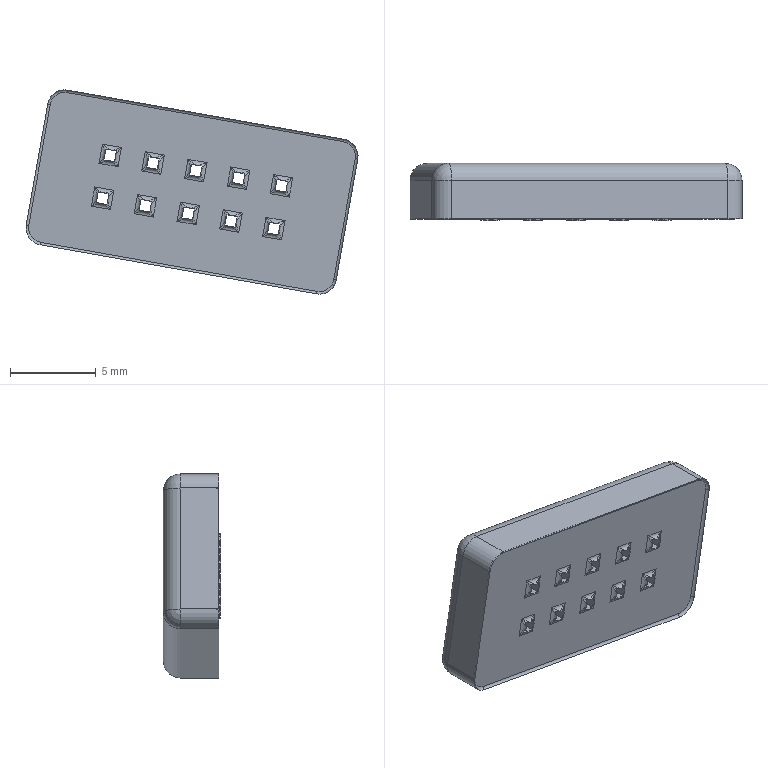Part | SolidWorks | features BaseBody 1 | 1 solid | 216 faces | box 19.402 x 3.35 x 11.935 mm | volume 493.088 mm3 | plane 86 | cylinder 82 | spline 40 | torus 4 | sphere 4 | commonest cylinder face diameters 0.5 x70 2 x8 0.3 x4